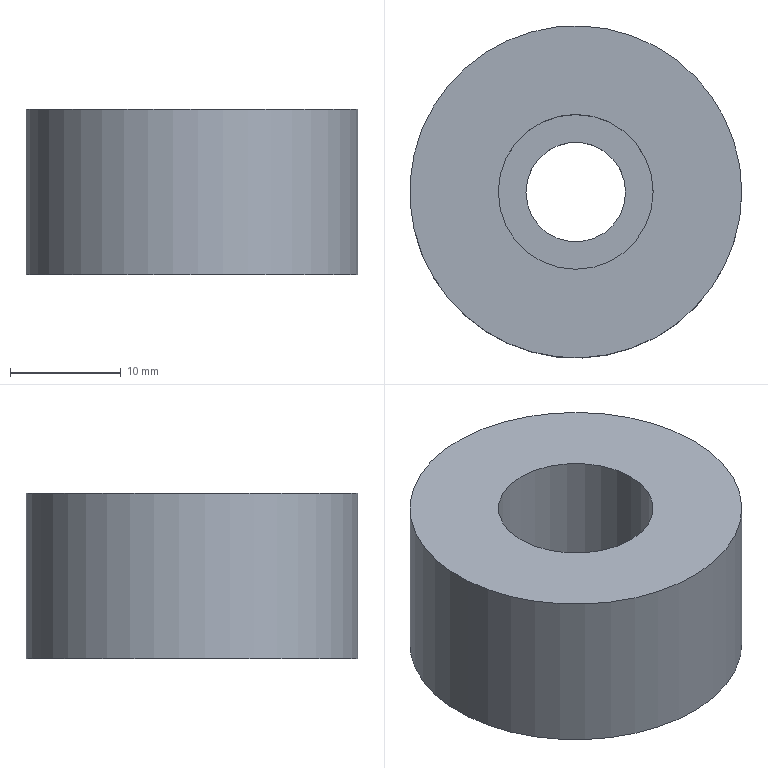Part | STEP file | 1 solid | 6 faces | box 30 x 30 x 15 mm | volume 8745 mm3 | plane 3 | cylinder 3 | commonest cylinder face diameters 9 x1 14 x1 30 x1
STEP:
#1=CARTESIAN_POINT('',(-318.,-75.,-32.));
#2=VERTEX_POINT('',#1);
#3=CARTESIAN_POINT('',(-325.,-75.,-32.));
#4=DIRECTION('',(0.,0.,-1.));
#5=DIRECTION('',(1.,0.,0.));
#6=AXIS2_PLACEMENT_3D('',#3,#4,#5);
#7=CIRCLE('',#6,7.);
#8=EDGE_CURVE('',#2,#2,#7,.T.);
#9=ORIENTED_EDGE('',*,*,#8,.T.);
#10=EDGE_LOOP('',(#9));
#11=FACE_BOUND('',#10,.T.);
#12=CARTESIAN_POINT('',(-310.,-75.,-32.));
#13=VERTEX_POINT('',#12);
#14=CARTESIAN_POINT('',(-325.,-75.,-32.));
#15=DIRECTION('',(0.,0.,-1.));
#16=DIRECTION('',(1.,0.,0.));
#17=AXIS2_PLACEMENT_3D('',#14,#15,#16);
#18=CIRCLE('',#17,15.);
#19=EDGE_CURVE('',#13,#13,#18,.T.);
#20=ORIENTED_EDGE('',*,*,#19,.F.);
#21=EDGE_LOOP('',(#20));
#22=FACE_BOUND('',#21,.T.);
#23=CARTESIAN_POINT('',(-325.,-75.,-32.));
#24=DIRECTION('',(0.,0.,1.));
#25=DIRECTION('',(1.,0.,0.));
#26=AXIS2_PLACEMENT_3D('',#23,#24,#25);
#27=PLANE('',#26);
#28=ADVANCED_FACE('',(#11,#22),#27,.T.);
#29=CARTESIAN_POINT('',(-320.5,-75.,-47.));
#30=VERTEX_POINT('',#29);
#31=CARTESIAN_POINT('',(-325.,-75.,-47.));
#32=DIRECTION('',(0.,0.,1.));
#33=DIRECTION('',(1.,0.,0.));
#34=AXIS2_PLACEMENT_3D('',#31,#32,#33);
#35=CIRCLE('',#34,4.5);
#36=EDGE_CURVE('',#30,#30,#35,.T.);
#37=ORIENTED_EDGE('',*,*,#36,.T.);
#38=EDGE_LOOP('',(#37));
#39=FACE_BOUND('',#38,.T.);
#40=CARTESIAN_POINT('',(-310.,-75.,-47.));
#41=VERTEX_POINT('',#40);
#42=CARTESIAN_POINT('',(-325.,-75.,-47.));
#43=DIRECTION('',(0.,0.,1.));
#44=DIRECTION('',(1.,0.,0.));
#45=AXIS2_PLACEMENT_3D('',#42,#43,#44);
#46=CIRCLE('',#45,15.);
#47=EDGE_CURVE('',#41,#41,#46,.T.);
#48=ORIENTED_EDGE('',*,*,#47,.F.);
#49=EDGE_LOOP('',(#48));
#50=FACE_BOUND('',#49,.T.);
#51=CARTESIAN_POINT('',(-325.,-75.,-47.));
#52=DIRECTION('',(0.,0.,-1.));
#53=DIRECTION('',(-1.,0.,0.));
#54=AXIS2_PLACEMENT_3D('',#51,#52,#53);
#55=PLANE('',#54);
#56=ADVANCED_FACE('',(#39,#50),#55,.T.);
#57=ORIENTED_EDGE('',*,*,#19,.T.);
#58=EDGE_LOOP('',(#57));
#59=FACE_BOUND('',#58,.T.);
#60=ORIENTED_EDGE('',*,*,#47,.T.);
#61=EDGE_LOOP('',(#60));
#62=FACE_BOUND('',#61,.T.);
#63=CARTESIAN_POINT('',(-325.,-75.,-47.));
#64=DIRECTION('',(0.,0.,1.));
#65=DIRECTION('',(1.,0.,0.));
#66=AXIS2_PLACEMENT_3D('',#63,#64,#65);
#67=CYLINDRICAL_SURFACE('',#66,15.);
#68=ADVANCED_FACE('',(#59,#62),#67,.T.);
#69=CARTESIAN_POINT('',(-329.5,-75.,-42.));
#70=VERTEX_POINT('',#69);
#71=CARTESIAN_POINT('',(-325.,-75.,-42.));
#72=DIRECTION('',(0.,0.,-1.));
#73=DIRECTION('',(-1.,0.,0.));
#74=AXIS2_PLACEMENT_3D('',#71,#72,#73);
#75=CIRCLE('',#74,4.5);
#76=EDGE_CURVE('',#70,#70,#75,.T.);
#77=ORIENTED_EDGE('',*,*,#76,.F.);
#78=EDGE_LOOP('',(#77));
#79=FACE_BOUND('',#78,.T.);
#80=ORIENTED_EDGE('',*,*,#36,.F.);
#81=EDGE_LOOP('',(#80));
#82=FACE_BOUND('',#81,.T.);
#83=CARTESIAN_POINT('',(-325.,-75.,-47.));
#84=DIRECTION('',(0.,0.,1.));
#85=DIRECTION('',(1.,0.,0.));
#86=AXIS2_PLACEMENT_3D('',#83,#84,#85);
#87=CYLINDRICAL_SURFACE('',#86,4.5);
#88=ADVANCED_FACE('',(#79,#82),#87,.F.);
#89=ORIENTED_EDGE('',*,*,#76,.T.);
#90=EDGE_LOOP('',(#89));
#91=FACE_BOUND('',#90,.T.);
#92=CARTESIAN_POINT('',(-318.,-75.,-42.));
#93=VERTEX_POINT('',#92);
#94=CARTESIAN_POINT('',(-325.,-75.,-42.));
#95=DIRECTION('',(0.,0.,-1.));
#96=DIRECTION('',(1.,0.,0.));
#97=AXIS2_PLACEMENT_3D('',#94,#95,#96);
#98=CIRCLE('',#97,7.);
#99=EDGE_CURVE('',#93,#93,#98,.T.);
#100=ORIENTED_EDGE('',*,*,#99,.F.);
#101=EDGE_LOOP('',(#100));
#102=FACE_BOUND('',#101,.T.);
#103=CARTESIAN_POINT('',(-325.,-75.,-42.));
#104=DIRECTION('',(0.,0.,-1.));
#105=DIRECTION('',(-1.,0.,0.));
#106=AXIS2_PLACEMENT_3D('',#103,#104,#105);
#107=PLANE('',#106);
#108=ADVANCED_FACE('',(#91,#102),#107,.F.);
#109=ORIENTED_EDGE('',*,*,#8,.F.);
#110=EDGE_LOOP('',(#109));
#111=FACE_BOUND('',#110,.T.);
#112=ORIENTED_EDGE('',*,*,#99,.T.);
#113=EDGE_LOOP('',(#112));
#114=FACE_BOUND('',#113,.T.);
#115=CARTESIAN_POINT('',(-325.,-75.,-42.));
#116=DIRECTION('',(0.,0.,1.));
#117=DIRECTION('',(1.,0.,0.));
#118=AXIS2_PLACEMENT_3D('',#115,#116,#117);
#119=CYLINDRICAL_SURFACE('',#118,7.);
#120=ADVANCED_FACE('',(#111,#114),#119,.F.);
#121=CLOSED_SHELL('',(#28,#56,#68,#88,#108,#120));
#122=MANIFOLD_SOLID_BREP('',#121);
#123=(LENGTH_UNIT()NAMED_UNIT(*)SI_UNIT(.MILLI.,.METRE.));
#124=UNCERTAINTY_MEASURE_WITH_UNIT(LENGTH_MEASURE(0.00002),#123,'','');
#125=(NAMED_UNIT(*)PLANE_ANGLE_UNIT()SI_UNIT($,.RADIAN.));
#126=PLANE_ANGLE_MEASURE_WITH_UNIT(PLANE_ANGLE_MEASURE(0.01745),#125);
#127=DIMENSIONAL_EXPONENTS(0.,0.,0.,0.,0.,0.,0.);
#128=(CONVERSION_BASED_UNIT('DEGREE',#126)NAMED_UNIT(#127)PLANE_ANGLE_UNIT());
#129=(NAMED_UNIT(*)SI_UNIT($,.STERADIAN.)SOLID_ANGLE_UNIT());
#130=(GEOMETRIC_REPRESENTATION_CONTEXT(3)GLOBAL_UNCERTAINTY_ASSIGNED_CONTEXT((#124))GLOBAL_UNIT_ASSIGNED_CONTEXT((#123,#128,#129))REPRESENTATION_CONTEXT('',''));
#131=ADVANCED_BREP_SHAPE_REPRESENTATION('',(#122),#130);